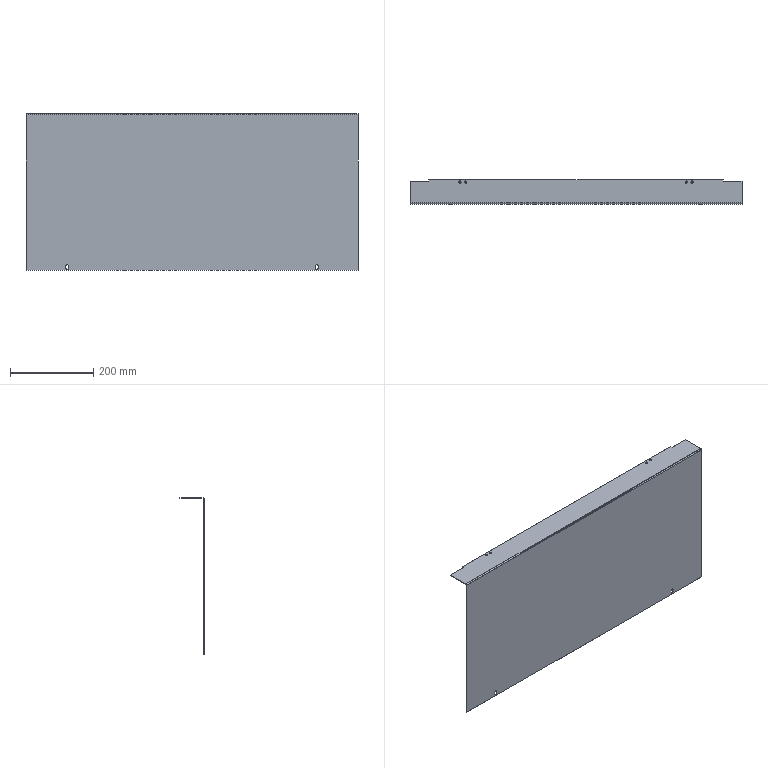Part | STEP file | Small busbar cover (flat top flange) | 1 solid | 36 faces | box 798 x 59 x 377 mm | volume 518069 mm3 | plane 20 | cylinder 16 | commonest cylinder face diameters 5.3 x8 7 x6 3 x1 6 x1